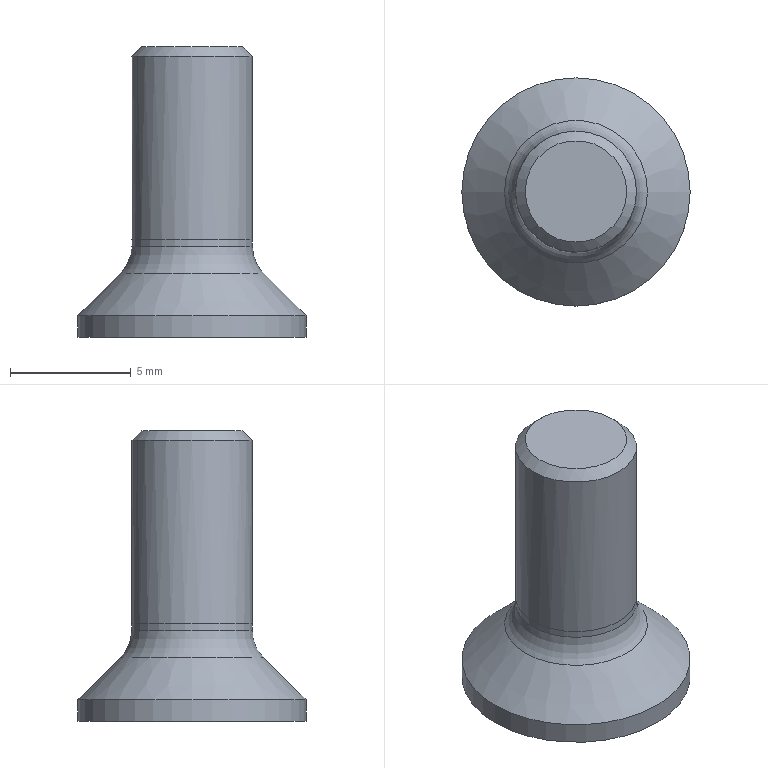Part | NX | features BREP 1 | 1 solid | 21 faces | box 9.43 x 9.43 x 12 mm | volume 313.297 mm3 | cone 9 | plane 8 | cylinder 3 | torus 1 | commonest cylinder face diameters 5 x2 9.43 x1
STEP:
#1=CARTESIAN_POINT('',(4.715,0.,0.));
#2=VERTEX_POINT('',#1);
#3=CARTESIAN_POINT('',(0.,0.,0.));
#4=DIRECTION('',(0.,0.,1.));
#5=DIRECTION('',(1.,0.,0.));
#6=AXIS2_PLACEMENT_3D('',#3,#4,#5);
#7=CIRCLE('',#6,4.715);
#8=EDGE_CURVE('',#2,#2,#7,.T.);
#9=ORIENTED_EDGE('',*,*,#8,.F.);
#10=EDGE_LOOP('',(#9));
#11=FACE_BOUND('',#10,.T.);
#12=CARTESIAN_POINT('',(1.5,0.866,0.));
#13=VERTEX_POINT('',#12);
#14=CARTESIAN_POINT('',(0.,1.732,0.));
#15=VERTEX_POINT('',#14);
#16=CARTESIAN_POINT('',(0.,0.,0.));
#17=DIRECTION('',(0.,0.,1.));
#18=DIRECTION('',(0.,1.,0.));
#19=AXIS2_PLACEMENT_3D('',#16,#17,#18);
#20=CIRCLE('',#19,1.732);
#21=EDGE_CURVE('',#13,#15,#20,.T.);
#22=ORIENTED_EDGE('',*,*,#21,.T.);
#23=CARTESIAN_POINT('',(-1.5,0.866,0.));
#24=VERTEX_POINT('',#23);
#25=CARTESIAN_POINT('',(0.,0.,0.));
#26=DIRECTION('',(0.,0.,1.));
#27=DIRECTION('',(0.,1.,0.));
#28=AXIS2_PLACEMENT_3D('',#25,#26,#27);
#29=CIRCLE('',#28,1.732);
#30=EDGE_CURVE('',#15,#24,#29,.T.);
#31=ORIENTED_EDGE('',*,*,#30,.T.);
#32=CARTESIAN_POINT('',(-1.5,-0.866,0.));
#33=VERTEX_POINT('',#32);
#34=CARTESIAN_POINT('',(0.,0.,0.));
#35=DIRECTION('',(0.,0.,1.));
#36=DIRECTION('',(0.,1.,0.));
#37=AXIS2_PLACEMENT_3D('',#34,#35,#36);
#38=CIRCLE('',#37,1.732);
#39=EDGE_CURVE('',#24,#33,#38,.T.);
#40=ORIENTED_EDGE('',*,*,#39,.T.);
#41=CARTESIAN_POINT('',(0.,-1.732,0.));
#42=VERTEX_POINT('',#41);
#43=CARTESIAN_POINT('',(0.,0.,0.));
#44=DIRECTION('',(0.,0.,1.));
#45=DIRECTION('',(0.,1.,0.));
#46=AXIS2_PLACEMENT_3D('',#43,#44,#45);
#47=CIRCLE('',#46,1.732);
#48=EDGE_CURVE('',#33,#42,#47,.T.);
#49=ORIENTED_EDGE('',*,*,#48,.T.);
#50=CARTESIAN_POINT('',(1.5,-0.866,0.));
#51=VERTEX_POINT('',#50);
#52=CARTESIAN_POINT('',(0.,0.,0.));
#53=DIRECTION('',(0.,0.,1.));
#54=DIRECTION('',(0.,1.,0.));
#55=AXIS2_PLACEMENT_3D('',#52,#53,#54);
#56=CIRCLE('',#55,1.732);
#57=EDGE_CURVE('',#42,#51,#56,.T.);
#58=ORIENTED_EDGE('',*,*,#57,.T.);
#59=CARTESIAN_POINT('',(0.,0.,0.));
#60=DIRECTION('',(0.,0.,1.));
#61=DIRECTION('',(0.,1.,0.));
#62=AXIS2_PLACEMENT_3D('',#59,#60,#61);
#63=CIRCLE('',#62,1.732);
#64=EDGE_CURVE('',#51,#13,#63,.T.);
#65=ORIENTED_EDGE('',*,*,#64,.T.);
#66=EDGE_LOOP('',(#22,#31,#40,#49,#58,#65));
#67=FACE_BOUND('',#66,.T.);
#68=CARTESIAN_POINT('',(0.,0.,0.));
#69=DIRECTION('',(0.,0.,1.));
#70=DIRECTION('',(1.,0.,0.));
#71=AXIS2_PLACEMENT_3D('',#68,#69,#70);
#72=PLANE('',#71);
#73=ADVANCED_FACE('',(#11,#67),#72,.F.);
#74=CARTESIAN_POINT('',(0.,1.732,0.));
#75=CARTESIAN_POINT('',(0.5357,1.423,0.1786));
#76=CARTESIAN_POINT('',(0.9639,1.176,0.1787));
#77=CARTESIAN_POINT('',(1.5,0.866,0.));
#78=B_SPLINE_CURVE_WITH_KNOTS('',3,(#74,#75,#76,#77),.UNSPECIFIED.,.F.,.F.,(4,4),(0.,1.),.UNSPECIFIED.);
#79=EDGE_CURVE('',#13,#15,#78,.F.);
#80=ORIENTED_EDGE('',*,*,#79,.T.);
#81=ORIENTED_EDGE('',*,*,#21,.F.);
#82=EDGE_LOOP('',(#80,#81));
#83=FACE_BOUND('',#82,.T.);
#84=CARTESIAN_POINT('',(0.,0.,0.));
#85=DIRECTION('',(0.,0.,-1.));
#86=DIRECTION('',(-1.,0.,0.));
#87=AXIS2_PLACEMENT_3D('',#84,#85,#86);
#88=CONICAL_SURFACE('',#87,1.732,1.047);
#89=ADVANCED_FACE('',(#83),#88,.F.);
#90=CARTESIAN_POINT('',(-1.5,0.866,0.));
#91=CARTESIAN_POINT('',(-0.9643,1.175,0.1786));
#92=CARTESIAN_POINT('',(-0.5361,1.423,0.1787));
#93=CARTESIAN_POINT('',(0.,1.732,0.));
#94=B_SPLINE_CURVE_WITH_KNOTS('',3,(#90,#91,#92,#93),.UNSPECIFIED.,.F.,.F.,(4,4),(0.,1.),.UNSPECIFIED.);
#95=EDGE_CURVE('',#15,#24,#94,.F.);
#96=ORIENTED_EDGE('',*,*,#95,.T.);
#97=ORIENTED_EDGE('',*,*,#30,.F.);
#98=EDGE_LOOP('',(#96,#97));
#99=FACE_BOUND('',#98,.T.);
#100=CARTESIAN_POINT('',(0.,0.,0.));
#101=DIRECTION('',(0.,0.,-1.));
#102=DIRECTION('',(-1.,0.,0.));
#103=AXIS2_PLACEMENT_3D('',#100,#101,#102);
#104=CONICAL_SURFACE('',#103,1.732,1.047);
#105=ADVANCED_FACE('',(#99),#104,.F.);
#106=CARTESIAN_POINT('',(-1.5,-0.866,0.));
#107=CARTESIAN_POINT('',(-1.5,-0.2474,0.1786));
#108=CARTESIAN_POINT('',(-1.5,0.247,0.1787));
#109=CARTESIAN_POINT('',(-1.5,0.866,0.));
#110=B_SPLINE_CURVE_WITH_KNOTS('',3,(#106,#107,#108,#109),.UNSPECIFIED.,.F.,.F.,(4,4),(0.,1.),.UNSPECIFIED.);
#111=EDGE_CURVE('',#24,#33,#110,.F.);
#112=ORIENTED_EDGE('',*,*,#111,.T.);
#113=ORIENTED_EDGE('',*,*,#39,.F.);
#114=EDGE_LOOP('',(#112,#113));
#115=FACE_BOUND('',#114,.T.);
#116=CARTESIAN_POINT('',(0.,0.,0.));
#117=DIRECTION('',(0.,0.,-1.));
#118=DIRECTION('',(-1.,0.,0.));
#119=AXIS2_PLACEMENT_3D('',#116,#117,#118);
#120=CONICAL_SURFACE('',#119,1.732,1.047);
#121=ADVANCED_FACE('',(#115),#120,.F.);
#122=CARTESIAN_POINT('',(0.,-1.732,0.));
#123=CARTESIAN_POINT('',(-0.5357,-1.423,0.1786));
#124=CARTESIAN_POINT('',(-0.9639,-1.176,0.1787));
#125=CARTESIAN_POINT('',(-1.5,-0.866,0.));
#126=B_SPLINE_CURVE_WITH_KNOTS('',3,(#122,#123,#124,#125),.UNSPECIFIED.,.F.,.F.,(4,4),(0.,1.),.UNSPECIFIED.);
#127=EDGE_CURVE('',#33,#42,#126,.F.);
#128=ORIENTED_EDGE('',*,*,#127,.T.);
#129=ORIENTED_EDGE('',*,*,#48,.F.);
#130=EDGE_LOOP('',(#128,#129));
#131=FACE_BOUND('',#130,.T.);
#132=CARTESIAN_POINT('',(0.,0.,0.));
#133=DIRECTION('',(0.,0.,-1.));
#134=DIRECTION('',(-1.,0.,0.));
#135=AXIS2_PLACEMENT_3D('',#132,#133,#134);
#136=CONICAL_SURFACE('',#135,1.732,1.047);
#137=ADVANCED_FACE('',(#131),#136,.F.);
#138=CARTESIAN_POINT('',(1.5,-0.866,0.));
#139=CARTESIAN_POINT('',(0.9643,-1.175,0.1786));
#140=CARTESIAN_POINT('',(0.5361,-1.423,0.1787));
#141=CARTESIAN_POINT('',(0.,-1.732,0.));
#142=B_SPLINE_CURVE_WITH_KNOTS('',3,(#138,#139,#140,#141),.UNSPECIFIED.,.F.,.F.,(4,4),(0.,1.),.UNSPECIFIED.);
#143=EDGE_CURVE('',#42,#51,#142,.F.);
#144=ORIENTED_EDGE('',*,*,#143,.T.);
#145=ORIENTED_EDGE('',*,*,#57,.F.);
#146=EDGE_LOOP('',(#144,#145));
#147=FACE_BOUND('',#146,.T.);
#148=CARTESIAN_POINT('',(0.,0.,0.));
#149=DIRECTION('',(0.,0.,-1.));
#150=DIRECTION('',(-1.,0.,0.));
#151=AXIS2_PLACEMENT_3D('',#148,#149,#150);
#152=CONICAL_SURFACE('',#151,1.732,1.047);
#153=ADVANCED_FACE('',(#147),#152,.F.);
#154=CARTESIAN_POINT('',(1.5,0.866,0.));
#155=CARTESIAN_POINT('',(1.5,0.2474,0.1786));
#156=CARTESIAN_POINT('',(1.5,-0.247,0.1787));
#157=CARTESIAN_POINT('',(1.5,-0.866,0.));
#158=B_SPLINE_CURVE_WITH_KNOTS('',3,(#154,#155,#156,#157),.UNSPECIFIED.,.F.,.F.,(4,4),(0.,1.),.UNSPECIFIED.);
#159=EDGE_CURVE('',#51,#13,#158,.F.);
#160=ORIENTED_EDGE('',*,*,#159,.T.);
#161=ORIENTED_EDGE('',*,*,#64,.F.);
#162=EDGE_LOOP('',(#160,#161));
#163=FACE_BOUND('',#162,.T.);
#164=CARTESIAN_POINT('',(0.,0.,0.));
#165=DIRECTION('',(0.,0.,-1.));
#166=DIRECTION('',(-1.,0.,0.));
#167=AXIS2_PLACEMENT_3D('',#164,#165,#166);
#168=CONICAL_SURFACE('',#167,1.732,1.047);
#169=ADVANCED_FACE('',(#163),#168,.F.);
#170=ORIENTED_EDGE('',*,*,#79,.F.);
#171=CARTESIAN_POINT('',(1.5,0.866,1.804));
#172=VERTEX_POINT('',#171);
#173=CARTESIAN_POINT('',(1.5,0.866,1.9));
#174=DIRECTION('',(0.,0.,-1.));
#175=VECTOR('',#174,1000.);
#176=LINE('',#173,#175);
#177=EDGE_CURVE('',#172,#13,#176,.T.);
#178=ORIENTED_EDGE('',*,*,#177,.F.);
#179=CARTESIAN_POINT('',(0.,1.732,1.804));
#180=VERTEX_POINT('',#179);
#181=CARTESIAN_POINT('',(1.5,0.866,1.804));
#182=CARTESIAN_POINT('',(1.,1.155,1.923));
#183=CARTESIAN_POINT('',(0.5,1.443,1.923));
#184=CARTESIAN_POINT('',(0.,1.732,1.804));
#185=B_SPLINE_CURVE_WITH_KNOTS('',3,(#181,#182,#183,#184),.UNSPECIFIED.,.F.,.F.,(4,4),(0.,1.),.UNSPECIFIED.);
#186=EDGE_CURVE('',#180,#172,#185,.F.);
#187=ORIENTED_EDGE('',*,*,#186,.F.);
#188=CARTESIAN_POINT('',(0.,1.732,1.9));
#189=DIRECTION('',(0.,0.,-1.));
#190=VECTOR('',#189,1000.);
#191=LINE('',#188,#190);
#192=EDGE_CURVE('',#180,#15,#191,.T.);
#193=ORIENTED_EDGE('',*,*,#192,.T.);
#194=EDGE_LOOP('',(#170,#178,#187,#193));
#195=FACE_BOUND('',#194,.T.);
#196=CARTESIAN_POINT('',(0.,1.732,1.9));
#197=DIRECTION('',(0.5,0.866,0.));
#198=DIRECTION('',(-0.866,0.5,0.));
#199=AXIS2_PLACEMENT_3D('',#196,#197,#198);
#200=PLANE('',#199);
#201=ADVANCED_FACE('',(#195),#200,.F.);
#202=ORIENTED_EDGE('',*,*,#95,.F.);
#203=ORIENTED_EDGE('',*,*,#192,.F.);
#204=CARTESIAN_POINT('',(-1.5,0.866,1.804));
#205=VERTEX_POINT('',#204);
#206=CARTESIAN_POINT('',(0.,1.732,1.804));
#207=CARTESIAN_POINT('',(-0.5,1.443,1.923));
#208=CARTESIAN_POINT('',(-1.,1.155,1.923));
#209=CARTESIAN_POINT('',(-1.5,0.866,1.804));
#210=B_SPLINE_CURVE_WITH_KNOTS('',3,(#206,#207,#208,#209),.UNSPECIFIED.,.F.,.F.,(4,4),(0.,1.),.UNSPECIFIED.);
#211=EDGE_CURVE('',#205,#180,#210,.F.);
#212=ORIENTED_EDGE('',*,*,#211,.F.);
#213=CARTESIAN_POINT('',(-1.5,0.866,1.9));
#214=DIRECTION('',(0.,0.,-1.));
#215=VECTOR('',#214,1000.);
#216=LINE('',#213,#215);
#217=EDGE_CURVE('',#205,#24,#216,.T.);
#218=ORIENTED_EDGE('',*,*,#217,.T.);
#219=EDGE_LOOP('',(#202,#203,#212,#218));
#220=FACE_BOUND('',#219,.T.);
#221=CARTESIAN_POINT('',(-1.5,0.866,1.9));
#222=DIRECTION('',(-0.5,0.866,0.));
#223=DIRECTION('',(-0.866,-0.5,0.));
#224=AXIS2_PLACEMENT_3D('',#221,#222,#223);
#225=PLANE('',#224);
#226=ADVANCED_FACE('',(#220),#225,.F.);
#227=ORIENTED_EDGE('',*,*,#111,.F.);
#228=ORIENTED_EDGE('',*,*,#217,.F.);
#229=CARTESIAN_POINT('',(-1.5,-0.866,1.804));
#230=VERTEX_POINT('',#229);
#231=CARTESIAN_POINT('',(-1.5,0.866,1.804));
#232=CARTESIAN_POINT('',(-1.5,0.2887,1.923));
#233=CARTESIAN_POINT('',(-1.5,-0.2887,1.923));
#234=CARTESIAN_POINT('',(-1.5,-0.866,1.804));
#235=B_SPLINE_CURVE_WITH_KNOTS('',3,(#231,#232,#233,#234),.UNSPECIFIED.,.F.,.F.,(4,4),(0.,1.),.UNSPECIFIED.);
#236=EDGE_CURVE('',#230,#205,#235,.F.);
#237=ORIENTED_EDGE('',*,*,#236,.F.);
#238=CARTESIAN_POINT('',(-1.5,-0.866,1.9));
#239=DIRECTION('',(0.,0.,-1.));
#240=VECTOR('',#239,1000.);
#241=LINE('',#238,#240);
#242=EDGE_CURVE('',#230,#33,#241,.T.);
#243=ORIENTED_EDGE('',*,*,#242,.T.);
#244=EDGE_LOOP('',(#227,#228,#237,#243));
#245=FACE_BOUND('',#244,.T.);
#246=CARTESIAN_POINT('',(-1.5,-0.866,1.9));
#247=DIRECTION('',(-1.,0.,0.));
#248=DIRECTION('',(0.,-1.,0.));
#249=AXIS2_PLACEMENT_3D('',#246,#247,#248);
#250=PLANE('',#249);
#251=ADVANCED_FACE('',(#245),#250,.F.);
#252=ORIENTED_EDGE('',*,*,#127,.F.);
#253=ORIENTED_EDGE('',*,*,#242,.F.);
#254=CARTESIAN_POINT('',(0.,-1.732,1.804));
#255=VERTEX_POINT('',#254);
#256=CARTESIAN_POINT('',(-1.5,-0.866,1.804));
#257=CARTESIAN_POINT('',(-1.,-1.155,1.923));
#258=CARTESIAN_POINT('',(-0.5,-1.443,1.923));
#259=CARTESIAN_POINT('',(0.,-1.732,1.804));
#260=B_SPLINE_CURVE_WITH_KNOTS('',3,(#256,#257,#258,#259),.UNSPECIFIED.,.F.,.F.,(4,4),(0.,1.),.UNSPECIFIED.);
#261=EDGE_CURVE('',#255,#230,#260,.F.);
#262=ORIENTED_EDGE('',*,*,#261,.F.);
#263=CARTESIAN_POINT('',(0.,-1.732,1.9));
#264=DIRECTION('',(0.,0.,-1.));
#265=VECTOR('',#264,1000.);
#266=LINE('',#263,#265);
#267=EDGE_CURVE('',#255,#42,#266,.T.);
#268=ORIENTED_EDGE('',*,*,#267,.T.);
#269=EDGE_LOOP('',(#252,#253,#262,#268));
#270=FACE_BOUND('',#269,.T.);
#271=CARTESIAN_POINT('',(0.,-1.732,1.9));
#272=DIRECTION('',(-0.5,-0.866,0.));
#273=DIRECTION('',(0.866,-0.5,0.));
#274=AXIS2_PLACEMENT_3D('',#271,#272,#273);
#275=PLANE('',#274);
#276=ADVANCED_FACE('',(#270),#275,.F.);
#277=ORIENTED_EDGE('',*,*,#143,.F.);
#278=ORIENTED_EDGE('',*,*,#267,.F.);
#279=CARTESIAN_POINT('',(1.5,-0.866,1.804));
#280=VERTEX_POINT('',#279);
#281=CARTESIAN_POINT('',(0.,-1.732,1.804));
#282=CARTESIAN_POINT('',(0.5,-1.443,1.923));
#283=CARTESIAN_POINT('',(1.,-1.155,1.923));
#284=CARTESIAN_POINT('',(1.5,-0.866,1.804));
#285=B_SPLINE_CURVE_WITH_KNOTS('',3,(#281,#282,#283,#284),.UNSPECIFIED.,.F.,.F.,(4,4),(0.,1.),.UNSPECIFIED.);
#286=EDGE_CURVE('',#280,#255,#285,.F.);
#287=ORIENTED_EDGE('',*,*,#286,.F.);
#288=CARTESIAN_POINT('',(1.5,-0.866,1.9));
#289=DIRECTION('',(0.,0.,-1.));
#290=VECTOR('',#289,1000.);
#291=LINE('',#288,#290);
#292=EDGE_CURVE('',#280,#51,#291,.T.);
#293=ORIENTED_EDGE('',*,*,#292,.T.);
#294=EDGE_LOOP('',(#277,#278,#287,#293));
#295=FACE_BOUND('',#294,.T.);
#296=CARTESIAN_POINT('',(1.5,-0.866,1.9));
#297=DIRECTION('',(0.5,-0.866,0.));
#298=DIRECTION('',(0.866,0.5,0.));
#299=AXIS2_PLACEMENT_3D('',#296,#297,#298);
#300=PLANE('',#299);
#301=ADVANCED_FACE('',(#295),#300,.F.);
#302=ORIENTED_EDGE('',*,*,#159,.F.);
#303=ORIENTED_EDGE('',*,*,#292,.F.);
#304=CARTESIAN_POINT('',(1.5,-0.866,1.804));
#305=CARTESIAN_POINT('',(1.5,-0.2887,1.923));
#306=CARTESIAN_POINT('',(1.5,0.2887,1.923));
#307=CARTESIAN_POINT('',(1.5,0.866,1.804));
#308=B_SPLINE_CURVE_WITH_KNOTS('',3,(#304,#305,#306,#307),.UNSPECIFIED.,.F.,.F.,(4,4),(0.,1.),.UNSPECIFIED.);
#309=EDGE_CURVE('',#172,#280,#308,.F.);
#310=ORIENTED_EDGE('',*,*,#309,.F.);
#311=ORIENTED_EDGE('',*,*,#177,.T.);
#312=EDGE_LOOP('',(#302,#303,#310,#311));
#313=FACE_BOUND('',#312,.T.);
#314=CARTESIAN_POINT('',(1.5,0.866,1.9));
#315=DIRECTION('',(1.,0.,0.));
#316=DIRECTION('',(0.,1.,0.));
#317=AXIS2_PLACEMENT_3D('',#314,#315,#316);
#318=PLANE('',#317);
#319=ADVANCED_FACE('',(#313),#318,.F.);
#320=CARTESIAN_POINT('',(0.,0.,2.521));
#321=VERTEX_POINT('',#320);
#322=VERTEX_LOOP('',#321);
#323=FACE_BOUND('',#322,.T.);
#324=ORIENTED_EDGE('',*,*,#286,.T.);
#325=ORIENTED_EDGE('',*,*,#261,.T.);
#326=ORIENTED_EDGE('',*,*,#236,.T.);
#327=ORIENTED_EDGE('',*,*,#211,.T.);
#328=ORIENTED_EDGE('',*,*,#186,.T.);
#329=ORIENTED_EDGE('',*,*,#309,.T.);
#330=EDGE_LOOP('',(#324,#325,#326,#327,#328,#329));
#331=FACE_BOUND('',#330,.T.);
#332=CARTESIAN_POINT('',(0.,0.,2.521));
#333=DIRECTION('',(0.,0.,-1.));
#334=DIRECTION('',(-1.,0.,0.));
#335=AXIS2_PLACEMENT_3D('',#332,#333,#334);
#336=CONICAL_SURFACE('',#335,0.,1.178);
#337=ADVANCED_FACE('',(#323,#331),#336,.F.);
#338=CARTESIAN_POINT('',(4.715,0.,0.885));
#339=VERTEX_POINT('',#338);
#340=CARTESIAN_POINT('',(0.,0.,0.885));
#341=DIRECTION('',(0.,0.,1.));
#342=DIRECTION('',(1.,0.,0.));
#343=AXIS2_PLACEMENT_3D('',#340,#341,#342);
#344=CIRCLE('',#343,4.715);
#345=EDGE_CURVE('',#339,#339,#344,.T.);
#346=ORIENTED_EDGE('',*,*,#345,.F.);
#347=EDGE_LOOP('',(#346));
#348=FACE_BOUND('',#347,.T.);
#349=ORIENTED_EDGE('',*,*,#8,.T.);
#350=EDGE_LOOP('',(#349));
#351=FACE_BOUND('',#350,.T.);
#352=CARTESIAN_POINT('',(0.,0.,20.));
#353=DIRECTION('',(0.,0.,1.));
#354=DIRECTION('',(1.,0.,0.));
#355=AXIS2_PLACEMENT_3D('',#352,#353,#354);
#356=CYLINDRICAL_SURFACE('',#355,4.715);
#357=ADVANCED_FACE('',(#348,#351),#356,.T.);
#358=CARTESIAN_POINT('',(2.5,0.,3.742));
#359=VERTEX_POINT('',#358);
#360=CARTESIAN_POINT('',(0.,0.,3.742));
#361=DIRECTION('',(0.,0.,1.));
#362=DIRECTION('',(1.,0.,0.));
#363=AXIS2_PLACEMENT_3D('',#360,#361,#362);
#364=CIRCLE('',#363,2.5);
#365=EDGE_CURVE('',#359,#359,#364,.T.);
#366=ORIENTED_EDGE('',*,*,#365,.F.);
#367=EDGE_LOOP('',(#366));
#368=FACE_BOUND('',#367,.T.);
#369=CARTESIAN_POINT('',(-2.954,0.,2.646));
#370=VERTEX_POINT('',#369);
#371=CARTESIAN_POINT('',(0.,0.,2.646));
#372=DIRECTION('',(0.,0.,-1.));
#373=DIRECTION('',(-1.,0.,0.));
#374=AXIS2_PLACEMENT_3D('',#371,#372,#373);
#375=CIRCLE('',#374,2.954);
#376=EDGE_CURVE('',#370,#370,#375,.T.);
#377=ORIENTED_EDGE('',*,*,#376,.F.);
#378=EDGE_LOOP('',(#377));
#379=FACE_BOUND('',#378,.T.);
#380=CARTESIAN_POINT('',(0.,0.,3.742));
#381=DIRECTION('',(0.,0.,1.));
#382=DIRECTION('',(1.,0.,0.));
#383=AXIS2_PLACEMENT_3D('',#380,#381,#382);
#384=TOROIDAL_SURFACE('',#383,4.05,1.55);
#385=ADVANCED_FACE('',(#368,#379),#384,.F.);
#386=CARTESIAN_POINT('',(-2.1,0.,12.));
#387=VERTEX_POINT('',#386);
#388=CARTESIAN_POINT('',(0.,0.,12.));
#389=DIRECTION('',(0.,0.,-1.));
#390=DIRECTION('',(-1.,0.,0.));
#391=AXIS2_PLACEMENT_3D('',#388,#389,#390);
#392=CIRCLE('',#391,2.1);
#393=EDGE_CURVE('',#387,#387,#392,.T.);
#394=ORIENTED_EDGE('',*,*,#393,.F.);
#395=EDGE_LOOP('',(#394));
#396=FACE_BOUND('',#395,.T.);
#397=CARTESIAN_POINT('',(2.5,0.,12.));
#398=DIRECTION('',(0.,0.,-1.));
#399=DIRECTION('',(-1.,0.,0.));
#400=AXIS2_PLACEMENT_3D('',#397,#398,#399);
#401=PLANE('',#400);
#402=ADVANCED_FACE('',(#396),#401,.F.);
#403=CARTESIAN_POINT('',(2.5,0.,11.6));
#404=VERTEX_POINT('',#403);
#405=CARTESIAN_POINT('',(0.,0.,11.6));
#406=DIRECTION('',(0.,0.,1.));
#407=DIRECTION('',(1.,0.,0.));
#408=AXIS2_PLACEMENT_3D('',#405,#406,#407);
#409=CIRCLE('',#408,2.5);
#410=EDGE_CURVE('',#404,#404,#409,.T.);
#411=ORIENTED_EDGE('',*,*,#410,.T.);
#412=EDGE_LOOP('',(#411));
#413=FACE_BOUND('',#412,.T.);
#414=ORIENTED_EDGE('',*,*,#393,.T.);
#415=EDGE_LOOP('',(#414));
#416=FACE_BOUND('',#415,.T.);
#417=CARTESIAN_POINT('',(0.,0.,11.6));
#418=DIRECTION('',(0.,0.,-1.));
#419=DIRECTION('',(-1.,0.,0.));
#420=AXIS2_PLACEMENT_3D('',#417,#418,#419);
#421=CONICAL_SURFACE('',#420,2.5,0.7854);
#422=ADVANCED_FACE('',(#413,#416),#421,.T.);
#423=CARTESIAN_POINT('',(2.5,0.,4.03));
#424=VERTEX_POINT('',#423);
#425=CARTESIAN_POINT('',(0.,0.,4.03));
#426=DIRECTION('',(0.,0.,1.));
#427=DIRECTION('',(1.,0.,0.));
#428=AXIS2_PLACEMENT_3D('',#425,#426,#427);
#429=CIRCLE('',#428,2.5);
#430=EDGE_CURVE('',#424,#424,#429,.T.);
#431=ORIENTED_EDGE('',*,*,#430,.F.);
#432=EDGE_LOOP('',(#431));
#433=FACE_BOUND('',#432,.T.);
#434=ORIENTED_EDGE('',*,*,#365,.T.);
#435=EDGE_LOOP('',(#434));
#436=FACE_BOUND('',#435,.T.);
#437=CARTESIAN_POINT('',(0.,0.,18.3));
#438=DIRECTION('',(0.,0.,1.));
#439=DIRECTION('',(1.,0.,0.));
#440=AXIS2_PLACEMENT_3D('',#437,#438,#439);
#441=CYLINDRICAL_SURFACE('',#440,2.5);
#442=ADVANCED_FACE('',(#433,#436),#441,.T.);
#443=ORIENTED_EDGE('',*,*,#410,.F.);
#444=EDGE_LOOP('',(#443));
#445=FACE_BOUND('',#444,.T.);
#446=ORIENTED_EDGE('',*,*,#430,.T.);
#447=EDGE_LOOP('',(#446));
#448=FACE_BOUND('',#447,.T.);
#449=CARTESIAN_POINT('',(0.,0.,18.3));
#450=DIRECTION('',(0.,0.,1.));
#451=DIRECTION('',(1.,0.,0.));
#452=AXIS2_PLACEMENT_3D('',#449,#450,#451);
#453=CYLINDRICAL_SURFACE('',#452,2.5);
#454=ADVANCED_FACE('',(#445,#448),#453,.T.);
#455=ORIENTED_EDGE('',*,*,#345,.T.);
#456=EDGE_LOOP('',(#455));
#457=FACE_BOUND('',#456,.T.);
#458=ORIENTED_EDGE('',*,*,#376,.T.);
#459=EDGE_LOOP('',(#458));
#460=FACE_BOUND('',#459,.T.);
#461=CARTESIAN_POINT('',(0.,0.,0.));
#462=DIRECTION('',(0.,0.,-1.));
#463=DIRECTION('',(-1.,0.,0.));
#464=AXIS2_PLACEMENT_3D('',#461,#462,#463);
#465=CONICAL_SURFACE('',#464,5.6,0.7854);
#466=ADVANCED_FACE('',(#457,#460),#465,.T.);
#467=CLOSED_SHELL('',(#73,#89,#105,#121,#137,#153,#169,#201,#226,#251,#276,#301,#319,#337,#357,#385,#402,#422,#442,#454,#466));
#468=MANIFOLD_SOLID_BREP('',#467);
#469=(LENGTH_UNIT()NAMED_UNIT(*)SI_UNIT(.MILLI.,.METRE.));
#470=UNCERTAINTY_MEASURE_WITH_UNIT(LENGTH_MEASURE(0.0508),#469,'','');
#471=(NAMED_UNIT(*)PLANE_ANGLE_UNIT()SI_UNIT($,.RADIAN.));
#472=(NAMED_UNIT(*)SI_UNIT($,.STERADIAN.)SOLID_ANGLE_UNIT());
#473=(GEOMETRIC_REPRESENTATION_CONTEXT(3)GLOBAL_UNCERTAINTY_ASSIGNED_CONTEXT((#470))GLOBAL_UNIT_ASSIGNED_CONTEXT((#469,#471,#472))REPRESENTATION_CONTEXT('',''));
#474=ADVANCED_BREP_SHAPE_REPRESENTATION('',(#468),#473);